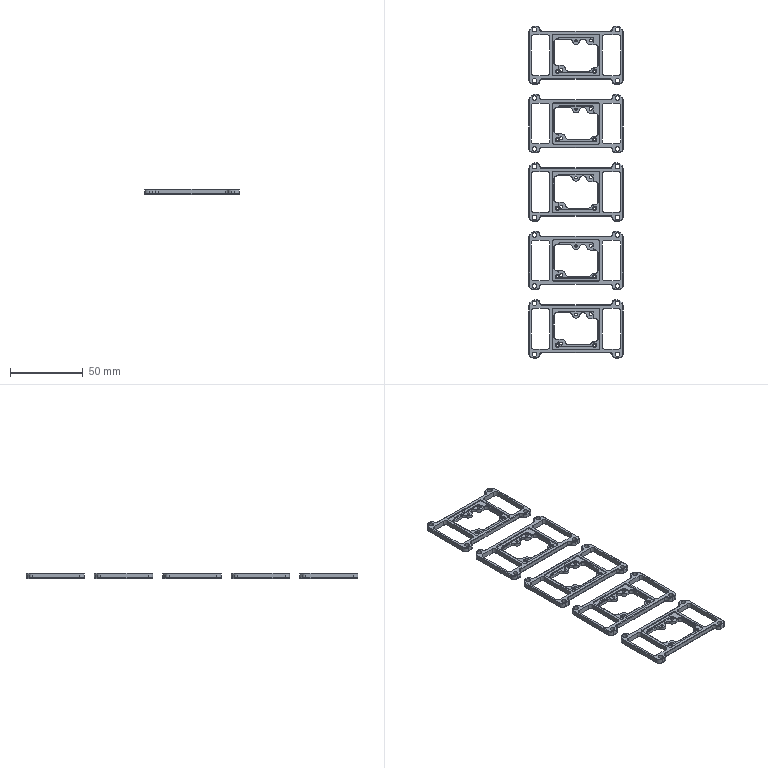NC program | NX | posted with a generic post | part box 65 x 228 x 3.5 mm
Lines 7047 to 8015 of 31259:
(ZLEVEL_PROFILE_COPY , TOOL : D4)
N14062 T04 M6
N14064 G54
N14066 G17 G0 G90 X-82.8 Y27.034 S9500 M3
N14068 G43 Z30. H4
N14070 Z0.2
N14072 G94 G1 Z-0.3 F1000.
N14074 X-82.2 Y27.38
N14076 G3 X-82. Y27.727 R0.4
N14078 G1 Y28.875 F1500.
N14080 X-83.148
N14082 G3 X-83.495 Y28.675 R0.4
N14084 G1 X-83.841 Y28.075
N14086 Z0.2
N14088 G0 X-82.8 Y27.034 Z-0.1
N14090 G1 Z-0.6 F1000.
N14092 X-82.2 Y27.38
N14094 G3 X-82. Y27.727 R0.4
N14096 G1 Y28.875 F1500.
N14098 X-83.148
N14100 G3 X-83.495 Y28.675 R0.4
N14102 G1 X-83.841 Y28.075
N14104 Z-0.1
N14106 G0 X-82.8 Y27.034 Z-0.4
N14108 G1 Z-0.9 F1000.
N14110 X-82.2 Y27.38
N14112 G3 X-82. Y27.727 R0.4
N14114 G1 Y28.875 F1500.
N14116 X-83.148
N14118 G3 X-83.495 Y28.675 R0.4
N14120 G1 X-83.841 Y28.075
N14122 Z-0.4
N14124 G0 X-82.8 Y27.034 Z-0.7
N14126 G1 Z-1.2 F1000.
N14128 X-82.2 Y27.38
N14130 G3 X-82. Y27.727 R0.4
N14132 G1 Y28.875 F1500.
N14134 X-83.148
N14136 G3 X-83.495 Y28.675 R0.4
N14138 G1 X-83.841 Y28.075
N14140 Z-0.7
N14142 G0 X-82.8 Y27.034 Z-1.
N14144 G1 Z-1.5 F1000.
N14146 X-82.2 Y27.38
N14148 G3 X-82. Y27.727 R0.4
N14150 G1 Y28.875 F1500.
N14152 X-83.148
N14154 G3 X-83.495 Y28.675 R0.4
N14156 G1 X-83.841 Y28.075
N14158 Z-1.
N14160 G0 X-82.8 Y27.034 Z-1.1
N14162 G1 Z-1.6 F1000.
N14164 X-82.2 Y27.38
N14166 G3 X-82. Y27.727 R0.4
N14168 G1 Y28.875 F1500.
N14170 X-83.148
N14172 G3 X-83.495 Y28.675 R0.4
N14174 G1 X-83.841 Y28.075
N14176 Z-1.1
N14178 G0 X-82.8 Y27.034 Z-1.48
N14180 G1 Z-1.98 F1000.
N14182 X-82.2 Y27.38
N14184 G3 X-82. Y27.727 R0.4
N14186 G1 Y28.875 F1500.
N14188 X-83.148
N14190 G3 X-83.495 Y28.675 R0.4
N14192 G1 X-83.841 Y28.075
N14194 Z-1.48
N14196 G0 X-82.8 Y27.034 Z-1.86
N14198 G1 Z-2.36 F1000.
N14200 X-82.2 Y27.38
N14202 G3 X-82. Y27.727 R0.4
N14204 G1 Y28.875 F1500.
N14206 X-83.148
N14208 G3 X-83.495 Y28.675 R0.4
N14210 G1 X-83.841 Y28.075
N14212 Z-1.86
N14214 G0 X-82.8 Y27.034 Z-2.24
N14216 G1 Z-2.74 F1000.
N14218 X-82.2 Y27.38
N14220 G3 X-82. Y27.727 R0.4
N14222 G1 Y28.875 F1500.
N14224 X-83.148
N14226 G3 X-83.495 Y28.675 R0.4
N14228 G1 X-83.841 Y28.075
N14230 Z-2.24
N14232 G0 X-82.8 Y27.034 Z-2.62
N14234 G1 Z-3.12 F1000.
N14236 X-82.2 Y27.38
N14238 G3 X-82. Y27.727 R0.4
N14240 G1 Y28.875 F1500.
N14242 X-83.148
N14244 G3 X-83.495 Y28.675 R0.4
N14246 G1 X-83.841 Y28.075
N14248 Z-2.62
N14250 G0 X-82.8 Y27.034 Z-3.
N14252 G1 Z-3.5 F1000.
N14254 X-82.2 Y27.38
N14256 G3 X-82. Y27.727 R0.4
N14258 G1 Y28.875 F1500.
N14260 X-83.148
N14262 G3 X-83.495 Y28.675 R0.4
N14264 G1 X-83.841 Y28.075
N14266 Z-3.
N14268 G0 Z10.
N14270 X-104.159
N14272 Z0.2
N14274 G1 Z-0.3 F1000.
N14276 X-104.505 Y28.675
N14278 G3 X-104.852 Y28.875 R0.4
N14280 G1 X-106. F1500.
N14282 Y27.727
N14284 G3 X-105.8 Y27.38 R0.4
N14286 G1 X-105.2 Y27.034
N14288 Z0.2
N14290 G0 X-104.159 Y28.075 Z-0.1
N14292 G1 Z-0.6 F1000.
N14294 X-104.505 Y28.675
N14296 G3 X-104.852 Y28.875 R0.4
N14298 G1 X-106. F1500.
N14300 Y27.727
N14302 G3 X-105.8 Y27.38 R0.4
N14304 G1 X-105.2 Y27.034
N14306 Z-0.1
N14308 G0 X-104.159 Y28.075 Z-0.4
N14310 G1 Z-0.9 F1000.
N14312 X-104.505 Y28.675
N14314 G3 X-104.852 Y28.875 R0.4
N14316 G1 X-106. F1500.
N14318 Y27.727
N14320 G3 X-105.8 Y27.38 R0.4
N14322 G1 X-105.2 Y27.034
N14324 Z-0.4
N14326 G0 X-104.159 Y28.075 Z-0.7
N14328 G1 Z-1.2 F1000.
N14330 X-104.505 Y28.675
N14332 G3 X-104.852 Y28.875 R0.4
N14334 G1 X-106. F1500.
N14336 Y27.727
N14338 G3 X-105.8 Y27.38 R0.4
N14340 G1 X-105.2 Y27.034
N14342 Z-0.7
N14344 G0 X-104.159 Y28.075 Z-1.
N14346 G1 Z-1.5 F1000.
N14348 X-104.505 Y28.675
N14350 G3 X-104.852 Y28.875 R0.4
N14352 G1 X-106. F1500.
N14354 Y27.727
N14356 G3 X-105.8 Y27.38 R0.4
N14358 G1 X-105.2 Y27.034
N14360 Z-1.
N14362 G0 X-104.159 Y28.075 Z-1.1
N14364 G1 Z-1.6 F1000.
N14366 X-104.505 Y28.675
N14368 G3 X-104.852 Y28.875 R0.4
N14370 G1 X-106. F1500.
N14372 Y27.727
N14374 G3 X-105.8 Y27.38 R0.4
N14376 G1 X-105.2 Y27.034
N14378 Z-1.1
N14380 G0 X-104.159 Y28.075 Z-1.48
N14382 G1 Z-1.98 F1000.
N14384 X-104.505 Y28.675
N14386 G3 X-104.852 Y28.875 R0.4
N14388 G1 X-106. F1500.
N14390 Y27.727
N14392 G3 X-105.8 Y27.38 R0.4
N14394 G1 X-105.2 Y27.034
N14396 Z-1.48
N14398 G0 X-104.159 Y28.075 Z-1.86
N14400 G1 Z-2.36 F1000.
N14402 X-104.505 Y28.675
N14404 G3 X-104.852 Y28.875 R0.4
N14406 G1 X-106. F1500.
N14408 Y27.727
N14410 G3 X-105.8 Y27.38 R0.4
N14412 G1 X-105.2 Y27.034
N14414 Z-1.86
N14416 G0 X-104.159 Y28.075 Z-2.24
N14418 G1 Z-2.74 F1000.
N14420 X-104.505 Y28.675
N14422 G3 X-104.852 Y28.875 R0.4
N14424 G1 X-106. F1500.
N14426 Y27.727
N14428 G3 X-105.8 Y27.38 R0.4
N14430 G1 X-105.2 Y27.034
N14432 Z-2.24
N14434 G0 X-104.159 Y28.075 Z-2.62
N14436 G1 Z-3.12 F1000.
N14438 X-104.505 Y28.675
N14440 G3 X-104.852 Y28.875 R0.4
N14442 G1 X-106. F1500.
N14444 Y27.727
N14446 G3 X-105.8 Y27.38 R0.4
N14448 G1 X-105.2 Y27.034
N14450 Z-2.62
N14452 G0 X-104.159 Y28.075 Z-3.
N14454 G1 Z-3.5 F1000.
N14456 X-104.505 Y28.675
N14458 G3 X-104.852 Y28.875 R0.4
N14460 G1 X-106. F1500.
N14462 Y27.727
N14464 G3 X-105.8 Y27.38 R0.4
N14466 G1 X-105.2 Y27.034
N14468 Z-3.
N14470 G0 Z10.
N14472 Y21.716
N14474 Z0.2
N14476 G1 Z-0.3 F1000.
N14478 X-105.8 Y21.37
N14480 G3 X-106. Y21.023 R0.4
N14482 G1 Y19.875 F1500.
N14484 X-104.852
N14486 G3 X-104.505 Y20.075 R0.4
N14488 G1 X-104.159 Y20.675
N14490 Z0.2
N14492 G0 X-105.2 Y21.716 Z-0.1
N14494 G1 Z-0.6 F1000.
N14496 X-105.8 Y21.37
N14498 G3 X-106. Y21.023 R0.4
N14500 G1 Y19.875 F1500.
N14502 X-104.852
N14504 G3 X-104.505 Y20.075 R0.4
N14506 G1 X-104.159 Y20.675
N14508 Z-0.1
N14510 G0 X-105.2 Y21.716 Z-0.4
N14512 G1 Z-0.9 F1000.
N14514 X-105.8 Y21.37
N14516 G3 X-106. Y21.023 R0.4
N14518 G1 Y19.875 F1500.
N14520 X-104.852
N14522 G3 X-104.505 Y20.075 R0.4
N14524 G1 X-104.159 Y20.675
N14526 Z-0.4
N14528 G0 X-105.2 Y21.716 Z-0.7
N14530 G1 Z-1.2 F1000.
N14532 X-105.8 Y21.37
N14534 G3 X-106. Y21.023 R0.4
N14536 G1 Y19.875 F1500.
N14538 X-104.852
N14540 G3 X-104.505 Y20.075 R0.4
N14542 G1 X-104.159 Y20.675
N14544 Z-0.7
N14546 G0 X-105.2 Y21.716 Z-1.
N14548 G1 Z-1.5 F1000.
N14550 X-105.8 Y21.37
N14552 G3 X-106. Y21.023 R0.4
N14554 G1 Y19.875 F1500.
N14556 X-104.852
N14558 G3 X-104.505 Y20.075 R0.4
N14560 G1 X-104.159 Y20.675
N14562 Z-1.
N14564 G0 X-105.2 Y21.716 Z-1.1
N14566 G1 Z-1.6 F1000.
N14568 X-105.8 Y21.37
N14570 G3 X-106. Y21.023 R0.4
N14572 G1 Y19.875 F1500.
N14574 X-104.852
N14576 G3 X-104.505 Y20.075 R0.4
N14578 G1 X-104.159 Y20.675
N14580 Z-1.1
N14582 G0 X-105.2 Y21.716 Z-1.48
N14584 G1 Z-1.98 F1000.
N14586 X-105.8 Y21.37
N14588 G3 X-106. Y21.023 R0.4
N14590 G1 Y19.875 F1500.
N14592 X-104.852
N14594 G3 X-104.505 Y20.075 R0.4
N14596 G1 X-104.159 Y20.675
N14598 Z-1.48
N14600 G0 X-105.2 Y21.716 Z-1.86
N14602 G1 Z-2.36 F1000.
N14604 X-105.8 Y21.37
N14606 G3 X-106. Y21.023 R0.4
N14608 G1 Y19.875 F1500.
N14610 X-104.852
N14612 G3 X-104.505 Y20.075 R0.4
N14614 G1 X-104.159 Y20.675
N14616 Z-1.86
N14618 G0 X-105.2 Y21.716 Z-2.24
N14620 G1 Z-2.74 F1000.
N14622 X-105.8 Y21.37
N14624 G3 X-106. Y21.023 R0.4
N14626 G1 Y19.875 F1500.
N14628 X-104.852
N14630 G3 X-104.505 Y20.075 R0.4
N14632 G1 X-104.159 Y20.675
N14634 Z-2.24
N14636 G0 X-105.2 Y21.716 Z-2.62
N14638 G1 Z-3.12 F1000.
N14640 X-105.8 Y21.37
N14642 G3 X-106. Y21.023 R0.4
N14644 G1 Y19.875 F1500.
N14646 X-104.852
N14648 G3 X-104.505 Y20.075 R0.4
N14650 G1 X-104.159 Y20.675
N14652 Z-2.62
N14654 G0 X-105.2 Y21.716 Z-3.
N14656 G1 Z-3.5 F1000.
N14658 X-105.8 Y21.37
N14660 G3 X-106. Y21.023 R0.4
N14662 G1 Y19.875 F1500.
N14664 X-104.852
N14666 G3 X-104.505 Y20.075 R0.4
N14668 G1 X-104.159 Y20.675
N14670 Z-3.
N14672 G0 Z10.
N14674 X-83.841
N14676 Z0.2
N14678 G1 Z-0.3 F1000.
N14680 X-83.495 Y20.075
N14682 G3 X-83.148 Y19.875 R0.4
N14684 G1 X-82.135 F1500.
N14686 X-81.997 Y19.872
N14688 X-82. Y19.917
N14690 Y21.023
N14692 G3 X-82.2 Y21.37 R0.4
N14694 G1 X-82.8 Y21.716
N14696 Z0.2
N14698 G0 X-83.841 Y20.675 Z-0.1
N14700 G1 Z-0.6 F1000.
N14702 X-83.495 Y20.075
N14704 G3 X-83.148 Y19.875 R0.4
N14706 G1 X-82.135 F1500.
N14708 X-81.997 Y19.872
N14710 X-82. Y21.023
N14712 G3 X-82.2 Y21.37 R0.4
N14714 G1 X-82.8 Y21.716
N14716 Z-0.1
N14718 G0 X-83.841 Y20.675 Z-0.4
N14720 G1 Z-0.9 F1000.
N14722 X-83.495 Y20.075
N14724 G3 X-83.148 Y19.875 R0.4
N14726 G1 X-82.135 F1500.
N14728 X-81.997 Y19.872
N14730 X-82. Y21.023
N14732 G3 X-82.2 Y21.37 R0.4
N14734 G1 X-82.8 Y21.716
N14736 Z-0.4
N14738 G0 X-83.841 Y20.675 Z-0.7
N14740 G1 Z-1.2 F1000.
N14742 X-83.495 Y20.075
N14744 G3 X-83.148 Y19.875 R0.4
N14746 G1 X-82.135 F1500.
N14748 X-81.998 Y19.873
N14750 X-82. Y21.023
N14752 G3 X-82.2 Y21.37 R0.4
N14754 G1 X-82.8 Y21.716
N14756 Z-0.7
N14758 G0 X-83.841 Y20.675 Z-1.
N14760 G1 Z-1.5 F1000.
N14762 X-83.495 Y20.075
N14764 G3 X-83.148 Y19.875 R0.4
N14766 G1 X-82.135 F1500.
N14768 X-81.998 Y19.873
N14770 X-82. Y21.023
N14772 G3 X-82.2 Y21.37 R0.4
N14774 G1 X-82.8 Y21.716
N14776 Z-1.
N14778 G0 X-83.841 Y20.675 Z-1.1
N14780 G1 Z-1.6 F1000.
N14782 X-83.495 Y20.075
N14784 G3 X-83.148 Y19.875 R0.4
N14786 G1 X-82.135 F1500.
N14788 X-81.998 Y19.873
N14790 X-82. Y21.023
N14792 G3 X-82.2 Y21.37 R0.4
N14794 G1 X-82.8 Y21.716
N14796 Z-1.1
N14798 G0 X-83.841 Y20.675 Z-1.48
N14800 G1 Z-1.98 F1000.
N14802 X-83.495 Y20.075
N14804 G3 X-83.148 Y19.875 R0.4
N14806 G1 X-82.135 F1500.
N14808 X-81.998 Y19.873
N14810 X-82. Y21.023
N14812 G3 X-82.2 Y21.37 R0.4
N14814 G1 X-82.8 Y21.716
N14816 Z-1.48
N14818 G0 X-83.841 Y20.675 Z-1.86
N14820 G1 Z-2.36 F1000.
N14822 X-83.495 Y20.075
N14824 G3 X-83.148 Y19.875 R0.4
N14826 G1 X-82.135 F1500.
N14828 X-81.999 Y19.874
N14830 X-82. Y21.023
N14832 G3 X-82.2 Y21.37 R0.4
N14834 G1 X-82.8 Y21.716
N14836 Z-1.86
N14838 G0 X-83.841 Y20.675 Z-2.24
N14840 G1 Z-2.74 F1000.
N14842 X-83.495 Y20.075
N14844 G3 X-83.148 Y19.875 R0.4
N14846 G1 X-82.135 F1500.
N14848 X-81.999 Y19.874
N14850 X-82. Y21.023
N14852 G3 X-82.2 Y21.37 R0.4
N14854 G1 X-82.8 Y21.716
N14856 Z-2.24
N14858 G0 X-83.841 Y20.675 Z-2.62
N14860 G1 Z-3.12 F1000.
N14862 X-83.495 Y20.075
N14864 G3 X-83.148 Y19.875 R0.4
N14866 G1 X-82. F1500.
N14868 Y21.023
N14870 G3 X-82.2 Y21.37 R0.4
N14872 G1 X-82.8 Y21.716
N14874 Z-2.62
N14876 G0 X-83.841 Y20.675 Z-3.
N14878 G1 Z-3.5 F1000.
N14880 X-83.495 Y20.075
N14882 G3 X-83.148 Y19.875 R0.4
N14884 G1 X-82. F1500.
N14886 Y21.023
N14888 G3 X-82.2 Y21.37 R0.4
N14890 G1 X-82.8 Y21.716
N14892 Z-3.
N14894 G0 Z10.
N14896 X-82.723 Y12.236
N14898 Z0.2
N14900 G1 Z-0.3 F1000.
N14902 X-82.123 Y12.582
N14904 G3 X-81.923 Y12.928 R0.4
N14906 G1 Y14.077 F1500.
N14908 X-83.072
N14910 G3 X-83.418 Y13.877 R0.4
N14912 G1 X-83.764 Y13.277
N14914 Z0.2
N14916 G0 X-82.75 Y12.209 Z-0.1
N14918 G1 Z-0.6 F1000.
N14920 X-82.15 Y12.555
N14922 G3 X-81.95 Y12.902 R0.4
N14924 G1 Y14.05 F1500.
N14926 X-83.098
N14928 G3 X-83.445 Y13.85 R0.4
N14930 G1 X-83.791 Y13.25
N14932 Z-0.1
N14934 G0 X-84.748 Y8.211 Z-0.4
N14936 G1 Z-0.9 F1000.
N14938 X-84.148 Y8.557
N14940 G3 X-83.948 Y8.903 R0.4
N14942 G1 Y10.137 F1500.
N14944 G2 X-84.591 Y10.052 R2.473
N14946 G1 X-85.097
N14948 G3 X-85.443 Y9.852 R0.4
N14950 G1 X-85.761 Y9.301
N14952 Z-0.4
N14954 G0 X-84.775 Y8.184 Z-0.7
N14956 G1 Z-1.2 F1000.
N14958 X-84.175 Y8.53
N14960 G3 X-83.975 Y8.877 R0.4
N14962 G1 Y10.102 F1500.
N14964 G2 X-84.591 Y10.025 R2.5
N14966 G1 X-85.123
N14968 G3 X-85.47 Y9.825 R0.4
N14970 G1 X-85.787 Y9.276
N14972 Z-0.7
N14974 G0 X-84.775 Y8.184 Z-1.
N14976 G1 Z-1.5 F1000.
N14978 X-84.175 Y8.53
N14980 G3 X-83.975 Y8.877 R0.4
N14982 G1 Y10.102 F1500.
N14984 G2 X-84.591 Y10.025 R2.5
N14986 G1 X-85.123
N14988 G3 X-85.47 Y9.825 R0.4
N14990 G1 X-85.787 Y9.276
N14992 Z-1.
N14994 G0 X-85.8 Y7.35 Z-1.1
N14996 G1 Z-1.6 F1000.
N14998 X-85.2 Y7.697
N15000 G3 X-85. Y8.043 R0.4
N15002 G1 Y8.747 F1500.
N15004 G2 X-85.574 Y9.118 R4.5
N15006 G3 X-85.971 Y9.169 R0.4
N15008 G1 X-86.565 Y8.92
N15010 Z-1.1
N15012 G0 X-85.8 Y7.35 Z-1.48
N15014 G1 Z-1.98 F1000.
N15016 X-85.2 Y7.697
N15018 G3 X-85. Y8.043 R0.4
N15020 G1 Y8.747 F1500.
N15022 G2 X-85.574 Y9.118 R4.5
N15024 G3 X-85.971 Y9.169 R0.4
N15026 G1 X-86.565 Y8.92
N15028 Z-1.48
N15030 G0 X-85.8 Y7.35 Z-1.86
N15032 G1 Z-2.36 F1000.
N15034 X-85.2 Y7.697
N15036 G3 X-85. Y8.043 R0.4
N15038 G1 Y8.747 F1500.
N15040 G2 X-85.574 Y9.118 R4.5
N15042 G3 X-85.971 Y9.169 R0.4
N15044 G1 X-86.565 Y8.92
N15046 Z-1.86
N15048 G0 X-85.8 Y7.35 Z-2.24
N15050 G1 Z-2.74 F1000.
N15052 X-85.2 Y7.697
N15054 G3 X-85. Y8.043 R0.4
N15056 G1 Y8.747 F1500.
N15058 G2 X-85.574 Y9.118 R4.5
N15060 G3 X-85.971 Y9.169 R0.4
N15062 G1 X-86.565 Y8.92
N15064 Z-2.24
N15066 G0 X-85.8 Y7.35 Z-2.62
N15068 G1 Z-3.12 F1000.
N15070 X-85.2 Y7.697
N15072 G3 X-85. Y8.043 R0.4
N15074 G1 Y8.747 F1500.
N15076 G2 X-85.574 Y9.118 R4.5
N15078 G3 X-85.971 Y9.169 R0.4
N15080 G1 X-86.565 Y8.92
N15082 Z-2.62
N15084 G0 X-85.8 Y7.35 Z-3.
N15086 G1 Z-3.5 F1000.
N15088 X-85.2 Y7.697
N15090 G3 X-85. Y8.043 R0.4
N15092 G1 Y8.747 F1500.
N15094 G2 X-85.574 Y9.118 R4.5
N15096 G3 X-85.971 Y9.169 R0.4
N15098 G1 X-86.565 Y8.92
N15100 Z-3.
N15102 G0 Z9.4
N15104 X-87.9 Y11.187
N15106 Z-0.4
N15108 G1 Z-0.9 F1000.
N15110 X-87.404 Y11.595
N15112 G3 X-87.263 Y11.969 R0.4
N15114 G2 X-87.313 Y12.998 R4.473 F1500.
N15116 G1 X-87.311 Y13.027
N15118 X-87.34
N15120 X-88.43
N15122 G3 X-88.776 Y12.827 R0.4
N15124 G1 X-89.123 Y12.227
N15126 Z-0.4
N15128 G0 X-87.921 Y11.162 Z-0.7
N15130 G1 Z-1.2 F1000.
N15132 X-87.426 Y11.572
N15134 G3 X-87.287 Y11.947 R0.4
N15136 G2 X-87.34 Y13. R4.5 F1500.
N15138 G1 X-88.454
N15140 G3 X-88.8 Y12.8 R0.4
N15142 G1 X-89.147 Y12.2
N15144 Z-0.7
N15146 G0 X-87.921 Y11.162 Z-1.
N15148 G1 Z-1.5 F1000.
N15150 X-87.426 Y11.572
N15152 G3 X-87.287 Y11.947 R0.4
N15154 G2 X-87.34 Y13. R4.5 F1500.
N15156 G1 X-88.454
N15158 G3 X-88.8 Y12.8 R0.4
N15160 G1 X-89.147 Y12.2
N15162 Z-1.
N15164 G0 X-87.922 Y11.161 Z-1.1
N15166 G1 Z-1.6 F1000.
N15168 X-87.426 Y11.572
N15170 G3 X-87.287 Y11.947 R0.4
N15172 G2 X-87.34 Y13. R4.5 F1500.
N15174 G1 X-88.454
N15176 G3 X-88.8 Y12.8 R0.4
N15178 G1 X-89.147 Y12.2
N15180 Z-1.1
N15182 G0 X-87.922 Y11.161 Z-1.48
N15184 G1 Z-1.98 F1000.
N15186 X-87.426 Y11.572
N15188 G3 X-87.287 Y11.947 R0.4
N15190 G2 X-87.34 Y13. R4.5 F1500.
N15192 G1 X-88.454
N15194 G3 X-88.8 Y12.8 R0.4
N15196 G1 X-89.147 Y12.2
N15198 Z-1.48
N15200 G0 X-87.922 Y11.161 Z-1.86
N15202 G1 Z-2.36 F1000.
N15204 X-87.426 Y11.572
N15206 G3 X-87.287 Y11.947 R0.4
N15208 G2 X-87.34 Y13. R4.5 F1500.
N15210 G1 X-88.454
N15212 G3 X-88.8 Y12.8 R0.4
N15214 G1 X-89.147 Y12.2
N15216 Z-1.86
N15218 G0 X-87.922 Y11.161 Z-2.24
N15220 G1 Z-2.74 F1000.
N15222 X-87.426 Y11.572
N15224 G3 X-87.287 Y11.947 R0.4
N15226 G2 X-87.34 Y13. R4.5 F1500.
N15228 G1 X-88.454
N15230 G3 X-88.8 Y12.8 R0.4
N15232 G1 X-89.147 Y12.2
N15234 Z-2.24
N15236 G0 X-87.922 Y11.161 Z-2.62
N15238 G1 Z-3.12 F1000.
N15240 X-87.426 Y11.572
N15242 G3 X-87.287 Y11.947 R0.4
N15244 G2 X-87.34 Y13. R4.5 F1500.
N15246 G1 X-88.454
N15248 G3 X-88.8 Y12.8 R0.4
N15250 G1 X-89.147 Y12.2
N15252 Z-2.62
N15254 G0 X-87.922 Y11.161 Z-3.
N15256 G1 Z-3.5 F1000.
N15258 X-87.426 Y11.572
N15260 G3 X-87.287 Y11.947 R0.4
N15262 G2 X-87.34 Y13. R4.5 F1500.
N15264 G1 X-88.454
N15266 G3 X-88.8 Y12.8 R0.4
N15268 G1 X-89.147 Y12.2
N15270 Z-3.
N15272 G0 Z10.
N15274 X-104.236 Y13.277
N15276 Z0.2
N15278 G1 Z-0.3 F1000.
N15280 X-104.582 Y13.877
N15282 G3 X-104.928 Y14.077 R0.4
N15284 G1 X-106.077 F1500.
N15286 Y12.928
N15288 G3 X-105.877 Y12.582 R0.4
N15290 G1 X-105.277 Y12.236
N15292 Z0.2
N15294 G0 X-104.209 Y13.25 Z-0.1
N15296 G1 Z-0.6 F1000.
N15298 X-104.555 Y13.85
N15300 G3 X-104.902 Y14.05 R0.4
N15302 G1 X-106.05 F1500.
N15304 Y12.902
N15306 G3 X-105.85 Y12.555 R0.4
N15308 G1 X-105.25 Y12.209
N15310 Z-0.1
N15312 G0 X-102.211 Y9.252 Z-0.4
N15314 G1 Z-0.9 F1000.
N15316 X-102.557 Y9.852
N15318 G3 X-102.903 Y10.052 R0.4
N15320 G1 X-104.052 F1500.
N15322 Y8.903
N15324 G3 X-103.852 Y8.557 R0.4
N15326 G1 X-103.252 Y8.211
N15328 Z-0.4
N15330 G0 X-102.184 Y9.225 Z-0.7
N15332 G1 Z-1.2 F1000.
N15334 X-102.53 Y9.825
N15336 G3 X-102.877 Y10.025 R0.4
N15338 G1 X-104.025 F1500.
N15340 Y8.877
N15342 G3 X-103.825 Y8.53 R0.4
N15344 G1 X-103.225 Y8.184
N15346 Z-0.7
N15348 G0 X-102.184 Y9.225 Z-1.
N15350 G1 Z-1.5 F1000.
N15352 X-102.53 Y9.825
N15354 G3 X-102.877 Y10.025 R0.4
N15356 G1 X-104.025 F1500.
N15358 Y8.877
N15360 G3 X-103.825 Y8.53 R0.4
N15362 G1 X-103.225 Y8.184
N15364 Z-1.
N15366 G0 X-100.584 Y5.487 Z-1.1
N15368 G1 Z-1.6 F1000.
N15370 X-101.149 Y5.805
N15372 G3 X-101.549 Y5.8 R0.4
N15374 G2 X-103. Y5.223 R5. F1500.
N15376 G1 Y4.419
N15378 G2 X-101.544 Y3.864 R4.5
N15380 G3 X-101.144 Y3.859 R0.4
N15382 G1 X-100.582 Y4.173
N15384 Z-1.1
N15386 G0 X-100.584 Y5.487 Z-1.48
N15388 G1 Z-1.98 F1000.
N15390 X-101.149 Y5.805
N15392 G3 X-101.549 Y5.8 R0.4
N15394 G2 X-103. Y5.223 R5. F1500.
N15396 G1 Y4.419
N15398 G2 X-101.544 Y3.864 R4.5
N15400 G3 X-101.144 Y3.859 R0.4
N15402 G1 X-100.582 Y4.173
N15404 Z-1.48
N15406 G0 X-100.584 Y5.487 Z-1.86
N15408 G1 Z-2.36 F1000.
N15410 X-101.149 Y5.805
N15412 G3 X-101.549 Y5.8 R0.4
N15414 G2 X-103. Y5.223 R5. F1500.
N15416 G1 Y4.419
N15418 G2 X-101.544 Y3.864 R4.5
N15420 G3 X-101.144 Y3.859 R0.4
N15422 G1 X-100.582 Y4.173
N15424 Z-1.86
N15426 G0 X-100.584 Y5.487 Z-2.24
N15428 G1 Z-2.74 F1000.
N15430 X-101.149 Y5.805
N15432 G3 X-101.549 Y5.8 R0.4
N15434 G2 X-103. Y5.223 R5. F1500.
N15436 G1 Y4.419
N15438 G2 X-101.544 Y3.864 R4.5
N15440 G3 X-101.144 Y3.859 R0.4
N15442 G1 X-100.582 Y4.173
N15444 Z-2.24
N15446 G0 X-100.584 Y5.487 Z-2.62
N15448 G1 Z-3.12 F1000.
N15450 X-101.149 Y5.805
N15452 G3 X-101.549 Y5.8 R0.4
N15454 G2 X-103. Y5.223 R5. F1500.
N15456 G1 Y4.419
N15458 G2 X-101.544 Y3.864 R4.5
N15460 G3 X-101.144 Y3.859 R0.4
N15462 G1 X-100.582 Y4.173
N15464 Z-2.62
N15466 G0 X-100.584 Y5.487 Z-3.
N15468 G1 Z-3.5 F1000.
N15470 X-101.149 Y5.805
N15472 G3 X-101.549 Y5.8 R0.4
N15474 G2 X-103. Y5.223 R5. F1500.
N15476 G1 Y4.419
N15478 G2 X-101.544 Y3.864 R4.5
N15480 G3 X-101.144 Y3.859 R0.4
N15482 G1 X-100.582 Y4.173
N15484 Z-3.
N15486 G0 Z9.4
N15488 X-97.321 Y12.227
N15490 Z-0.4
N15492 G1 Z-0.9 F1000.
N15494 X-97.668 Y12.827
N15496 G3 X-98.014 Y13.027 R0.4
N15498 G1 X-99.1 F1500.
N15500 X-99.128 Y13.028
N15502 X-99.127 Y13.
N15504 Y12.525
N15506 G2 X-99.19 Y11.97 R2.473
N15508 G3 X-99.073 Y11.587 R0.4
N15510 G1 X-98.622 Y11.167
N15512 Z-0.4
N15514 G0 X-97.298 Y12.2 Z-0.7
N15516 G1 Z-1.2 F1000.
N15518 X-97.645 Y12.8
N15520 G3 X-97.991 Y13. R0.4
N15522 G1 X-99.1 F1500.
N15524 Y12.525
N15526 G2 X-99.167 Y11.95 R2.5
N15528 G3 X-99.052 Y11.567 R0.4
N15530 G1 X-98.603 Y11.144
N15532 Z-0.7
N15534 G0 X-97.298 Y12.2 Z-1.
N15536 G1 Z-1.5 F1000.
N15538 X-97.645 Y12.8
N15540 G3 X-97.991 Y13. R0.4
N15542 G1 X-99.1 F1500.
N15544 Y12.525
N15546 G2 X-99.167 Y11.95 R2.5
N15548 G3 X-99.052 Y11.567 R0.4
N15550 G1 X-98.603 Y11.144
N15552 Z-1.
N15554 G0 X-97.259 Y12.2 Z-1.1
N15556 G1 Z-1.6 F1000.
N15558 X-97.605 Y12.8
N15560 G3 X-97.952 Y13. R0.4
N15562 G1 X-99.1 F1500.
N15564 Y11.852
N15566 G3 X-98.9 Y11.505 R0.4
N15568 G1 X-98.3 Y11.159
N15570 Z-1.1
N15572 G0 X-97.259 Y12.2 Z-1.48
N15574 G1 Z-1.98 F1000.
N15576 X-97.605 Y12.8
N15578 G3 X-97.952 Y13. R0.4
N15580 G1 X-99.1 F1500.
N15582 Y11.852
N15584 G3 X-98.9 Y11.505 R0.4
N15586 G1 X-98.3 Y11.159
N15588 Z-1.48
N15590 G0 X-97.259 Y12.2 Z-1.86
N15592 G1 Z-2.36 F1000.
N15594 X-97.605 Y12.8
N15596 G3 X-97.952 Y13. R0.4
N15598 G1 X-99.1 F1500.
N15600 Y11.852
N15602 G3 X-98.9 Y11.505 R0.4
N15604 G1 X-98.3 Y11.159
N15606 Z-1.86
N15608 G0 X-97.259 Y12.2 Z-2.24
N15610 G1 Z-2.74 F1000.
N15612 X-97.605 Y12.8
N15614 G3 X-97.952 Y13. R0.4
N15616 G1 X-99.1 F1500.
N15618 Y11.852
N15620 G3 X-98.9 Y11.505 R0.4
N15622 G1 X-98.3 Y11.159
N15624 Z-2.24
N15626 G0 X-97.259 Y12.2 Z-2.62
N15628 G1 Z-3.12 F1000.
N15630 X-97.605 Y12.8
N15632 G3 X-97.952 Y13. R0.4
N15634 G1 X-99.1 F1500.
N15636 Y11.852
N15638 G3 X-98.9 Y11.505 R0.4
N15640 G1 X-98.3 Y11.159
N15642 Z-2.62
N15644 G0 X-97.259 Y12.2 Z-3.
N15646 G1 Z-3.5 F1000.
N15648 X-97.605 Y12.8
N15650 G3 X-97.952 Y13. R0.4
N15652 G1 X-99.1 F1500.
N15654 Y11.852
N15656 G3 X-98.9 Y11.505 R0.4
N15658 G1 X-98.3 Y11.159
N15660 Z-3.
N15662 G0 Z10.
N15664 X-105.277 Y-12.236
N15666 Z0.2
N15668 G1 Z-0.3 F1000.
N15670 X-105.877 Y-12.582
N15672 G3 X-106.077 Y-12.928 R0.4
N15674 G1 Y-14.077 F1500.
N15676 X-104.928
N15678 G3 X-104.582 Y-13.877 R0.4
N15680 G1 X-104.236 Y-13.277
N15682 Z0.2
N15684 G0 X-105.25 Y-12.209 Z-0.1
N15686 G1 Z-0.6 F1000.
N15688 X-105.85 Y-12.555
N15690 G3 X-106.05 Y-12.902 R0.4
N15692 G1 Y-14.05 F1500.
N15694 X-104.902
N15696 G3 X-104.555 Y-13.85 R0.4
N15698 G1 X-104.209 Y-13.25
N15700 Z-0.1
N15702 G0 X-102.37 Y-11.169 Z-0.4
N15704 G1 Z-0.9 F1000.
N15706 X-102.865 Y-11.515
N15708 G3 X-103.034 Y-11.878 R0.4
N15710 G1 X-103.027 Y-12.052 F1500.
N15712 Y-13.
N15714 X-103.028 Y-13.028
N15716 X-103. Y-13.027
N15718 X-101.878
N15720 G3 X-101.532 Y-12.827 R0.4
N15722 G1 X-101.185 Y-12.227
N15724 Z-0.4
N15726 G0 X-102.343 Y-11.143 Z-0.7
N15728 G1 Z-1.2 F1000.
N15730 X-102.838 Y-11.489
N15732 G3 X-103.008 Y-11.852 R0.4
N15734 G1 X-103. Y-12.025 F1500.
N15736 Y-13.
N15738 X-101.852
N15740 G3 X-101.505 Y-12.8 R0.4
N15742 G1 X-101.159 Y-12.2
N15744 Z-0.7
N15746 G0 X-102.343 Y-11.143 Z-1.
N15748 G1 Z-1.5 F1000.
N15750 X-102.838 Y-11.489
N15752 G3 X-103.008 Y-11.852 R0.4
N15754 G1 X-103. Y-12.025 F1500.
N15756 Y-13.
N15758 X-101.852
N15760 G3 X-101.505 Y-12.8 R0.4
N15762 G1 X-101.159 Y-12.2
N15764 Z-1.
N15766 G0 X-102.2 Y-11.159 Z-1.1
N15768 G1 Z-1.6 F1000.
N15770 X-102.8 Y-11.505
N15772 G3 X-103. Y-11.852 R0.4
N15774 G1 Y-13. F1500.
N15776 X-101.852
N15778 G3 X-101.505 Y-12.8 R0.4
N15780 G1 X-101.159 Y-12.2
N15782 Z-1.1
N15784 G0 X-102.2 Y-11.159 Z-1.48
N15786 G1 Z-1.98 F1000.
N15788 X-102.8 Y-11.505
N15790 G3 X-103. Y-11.852 R0.4
N15792 G1 Y-13. F1500.
N15794 X-101.852
N15796 G3 X-101.505 Y-12.8 R0.4
N15798 G1 X-101.159 Y-12.2
N15800 Z-1.48
N15802 G0 X-102.2 Y-11.159 Z-1.86
N15804 G1 Z-2.36 F1000.
N15806 X-102.8 Y-11.505
N15808 G3 X-103. Y-11.852 R0.4
N15810 G1 Y-13. F1500.
N15812 X-101.852
N15814 G3 X-101.505 Y-12.8 R0.4
N15816 G1 X-101.159 Y-12.2
N15818 Z-1.86
N15820 G0 X-102.2 Y-11.159 Z-2.24
N15822 G1 Z-2.74 F1000.
N15824 X-102.8 Y-11.505
N15826 G3 X-103. Y-11.852 R0.4
N15828 G1 Y-13. F1500.
N15830 X-101.852
N15832 G3 X-101.505 Y-12.8 R0.4
N15834 G1 X-101.159 Y-12.2
N15836 Z-2.24
N15838 G0 X-102.2 Y-11.159 Z-2.62
N15840 G1 Z-3.12 F1000.
N15842 X-102.8 Y-11.505
N15844 G3 X-103. Y-11.852 R0.4
N15846 G1 Y-13. F1500.
N15848 X-101.852
N15850 G3 X-101.505 Y-12.8 R0.4
N15852 G1 X-101.159 Y-12.2
N15854 Z-2.62
N15856 G0 X-102.2 Y-11.159 Z-3.
N15858 G1 Z-3.5 F1000.
N15860 X-102.8 Y-11.505
N15862 G3 X-103. Y-11.852 R0.4
N15864 G1 Y-13. F1500.
N15866 X-101.852
N15868 G3 X-101.505 Y-12.8 R0.4
N15870 G1 X-101.159 Y-12.2
N15872 Z-3.
N15874 G0 Z9.4
N15876 X-103.252 Y-8.964
N15878 Z-0.4
N15880 G1 Z-0.9 F1000.
N15882 X-103.852 Y-9.311
N15884 G3 X-104.052 Y-9.657 R0.4
N15886 G1 Y-10.305 F1500.
N15888 G2 X-103.568 Y-10.684 R2.001
N15890 G3 X-103.185 Y-10.8 R0.4
N15892 G1 X-102.596 Y-10.662
N15894 Z-0.4
N15896 G0 X-103.225 Y-8.926 Z-0.7
N15898 G1 Z-1.2 F1000.
N15900 X-103.825 Y-9.272
N15902 G3 X-104.025 Y-9.618 R0.4
N15904 G1 Y-10.279 F1500.
N15906 G2 X-103.53 Y-10.669 R2.
N15908 G3 X-103.148 Y-10.788 R0.4
N15910 G1 X-102.558 Y-10.655
N15912 Z-0.7
N15914 G0 X-103.225 Y-8.926 Z-1.
N15916 G1 Z-1.5 F1000.
N15918 X-103.825 Y-9.272
N15920 G3 X-104.025 Y-9.618 R0.4
N15922 G1 Y-10.279 F1500.
N15924 G2 X-103.53 Y-10.669 R2.
N15926 G3 X-103.148 Y-10.788 R0.4
N15928 G1 X-102.558 Y-10.655
N15930 Z-1.
N15932 G0 X-101.262 Y-4.625 Z-1.1
N15934 G1 Z-1.6 F1000.
N15936 X-101.77 Y-4.229
N15938 G3 X-102.166 Y-4.173 R0.4
N15940 G2 X-103. Y-4.419 R4.5 F1500.
N15942 G1 Y-5.328
N15944 G3 X-102.8 Y-5.674 R0.4
N15946 G1 X-102.2 Y-6.021
N15948 Z-1.1
N15950 G0 X-101.262 Y-4.625 Z-1.48
N15952 G1 Z-1.98 F1000.
N15954 X-101.77 Y-4.229
N15956 G3 X-102.166 Y-4.173 R0.4
N15958 G2 X-103. Y-4.419 R4.5 F1500.
N15960 G1 Y-5.328
N15962 G3 X-102.8 Y-5.674 R0.4
N15964 G1 X-102.2 Y-6.021
N15966 Z-1.48
N15968 G0 X-101.262 Y-4.625 Z-1.86
N15970 G1 Z-2.36 F1000.
N15972 X-101.77 Y-4.229
N15974 G3 X-102.166 Y-4.173 R0.4
N15976 G2 X-103. Y-4.419 R4.5 F1500.
N15978 G1 Y-5.328
N15980 G3 X-102.8 Y-5.674 R0.4
N15982 G1 X-102.2 Y-6.021
N15984 Z-1.86
N15986 G0 X-101.262 Y-4.625 Z-2.24
N15988 G1 Z-2.74 F1000.
N15990 X-101.77 Y-4.229
N15992 G3 X-102.166 Y-4.173 R0.4